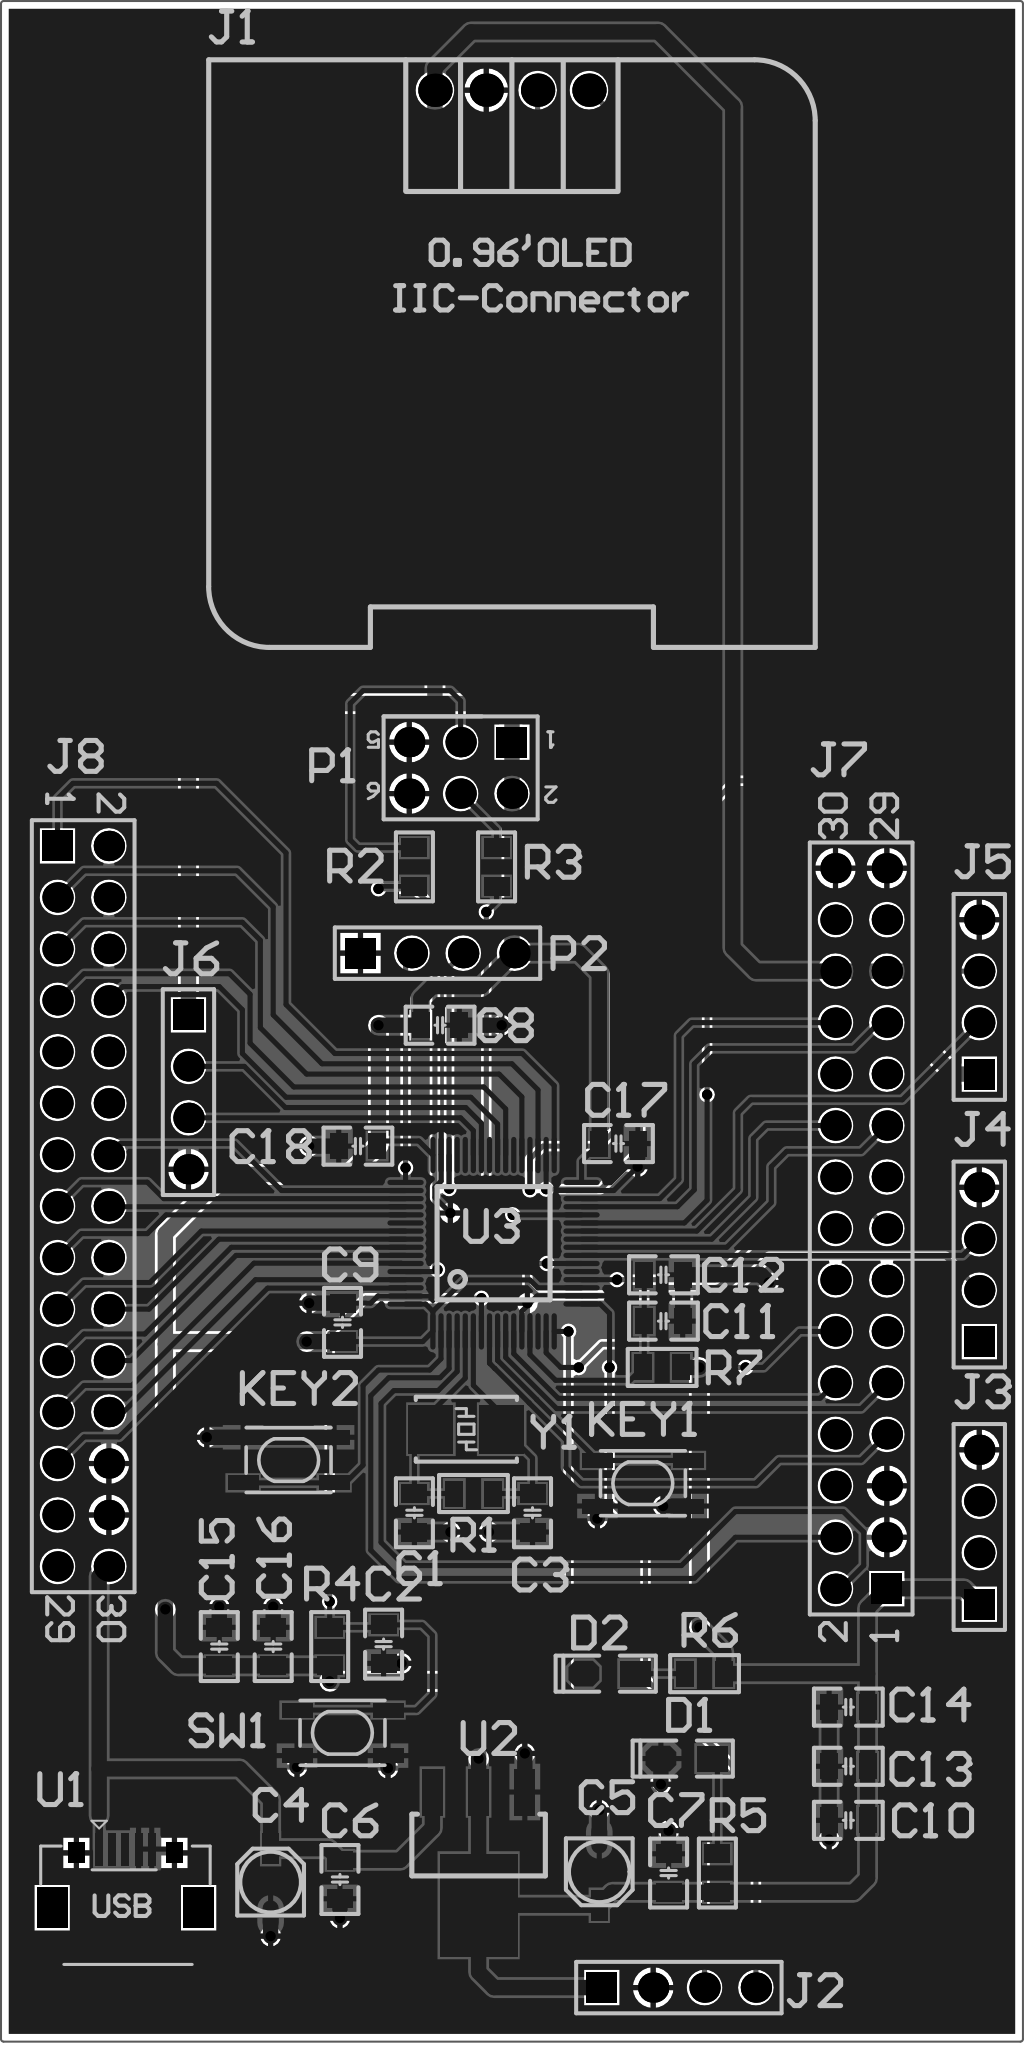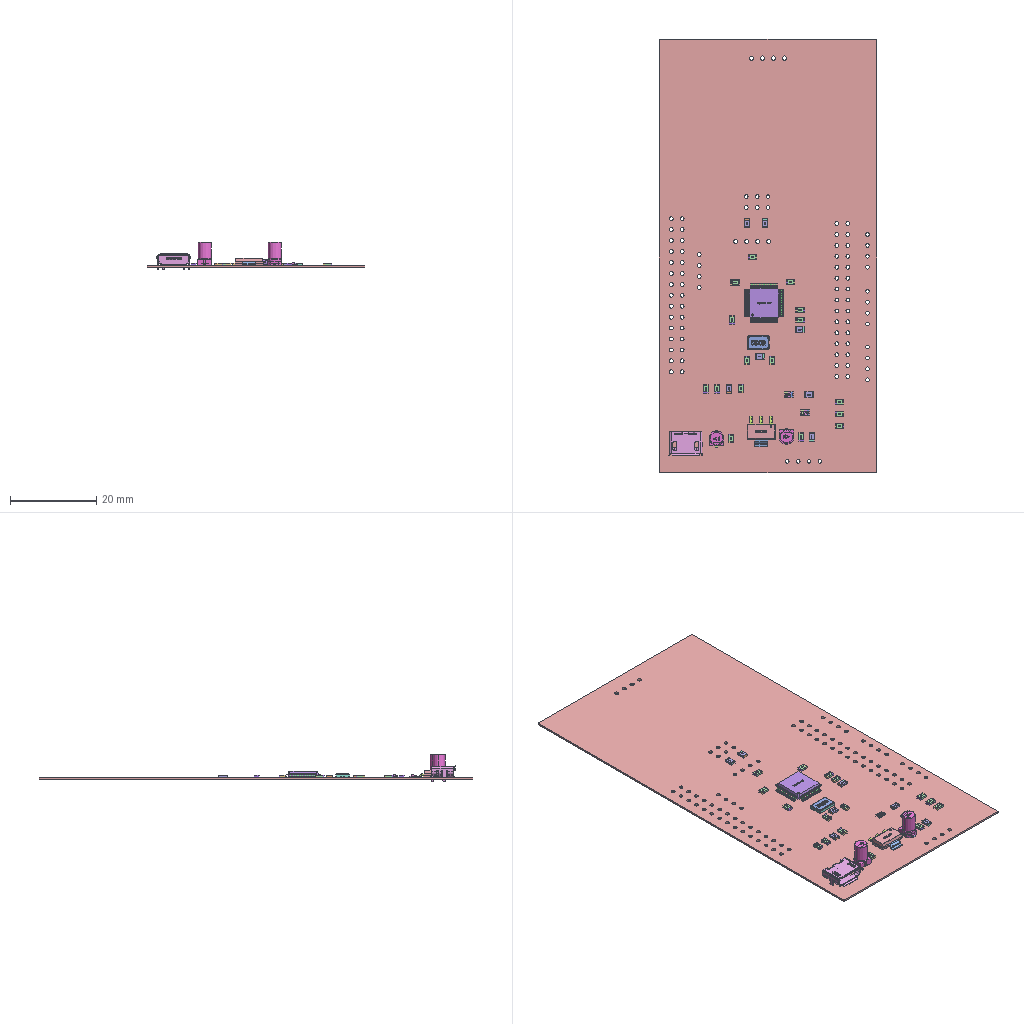Circuit board layout | Altium Designer | box 50.5 x 100.7 x 6.4 mm
Layer stack:
# Altium Designer layer stack of  (unit mm; dielectric type: 0 none, 1 core, 2 prepreg, 3 surface material)
index,name,kind,layer,copper_thickness_mm,dielectric_type,dielectric_thickness_mm,dielectric_material,dielectric_constant
0,Top Paste,other,,,,,,
1,Top Overlay,other,,,,,,
2,Top Solder,dielectric,,,3,0.0102,Solder Resist,3.5
3,Top Layer,copper,Top Layer,0.0356,,,,
4,Dielectric 1,dielectric,,,0,0.32,FR-4,4.8
5,Bottom Layer,copper,Bottom Layer,0.0356,,,,
6,Bottom Solder,dielectric,,,3,0.0102,Solder Resist,3.5
7,Bottom Overlay,other,,,,,,
8,Bottom Paste,other,,,,,,
# drill layer pairs: low layer,high layer
drill_pair,Top Layer,Bottom Layer
Part placement:
Designator,Comment,Layer,Footprint,Center-X(mm),Center-Y(mm),Rotation
Y1,8M,TopLayer,OSC_5032-2P,74.323,63.881,180
U3,STM32F103RCT6,TopLayer,LQFP64_7x7,75.67,73.059,0
U2,AMS1117-3.3,TopLayer,SOT223,74.93,43.18,180
U1,USB-Micro,TopLayer,USB-MICRO_B,57.462,41.709,0
SW1,SW-PB,TopLayer,TSW_SMD-3*4*2.5,68.199,48.895,180
R7,Res2,TopLayer,R_0805_L,84.008,66.929,180
R6,Res1,TopLayer,R_0805_L,86.106,51.816,180
R5,Res1,TopLayer,R_0805_L,86.741,41.976,90
R4,Res2,TopLayer,R_0805_L,67.564,53.152,270
R3,Res2,TopLayer,R_0805_L,75.819,91.633,270
R2,Res2,TopLayer,R_0805_L,71.755,91.633,90
R1,,TopLayer,R_0805_L,74.676,60.706,180
P2,SWD,TopLayer,HDR1X4,72.898,87.376,360
P1,Header 3X2,TopLayer,HDR2X3,74.041,96.52,180
KEY2,SW-PB,TopLayer,TSW_SMD-3*4*2.5,65.532,62.357,360
KEY1,SW-PB,TopLayer,TSW_SMD-3*4*2.5,83.058,61.214,180
J8,HEADER 15X2,TopLayer,HDR2X15,55.372,74.887,270
J7,HEADER 15X2,TopLayer,HDR2X15,93.853,73.787,90
J6,HC-SR04,TopLayer,HDR1X4,60.579,80.518,270
J5,HC-SR04,TopLayer,HDR1X4,99.695,85.217,90
J4,HC-SR04,TopLayer,HDR1X4,99.695,72.009,90
J3,HC-SR04,TopLayer,HDR1X4,99.695,59.055,90
J2,SIM900A,TopLayer,HDR1X4,84.836,36.322,360
J1,OLED,TopLayer,0.96OLED_4P,76.58,129.966,0
D2,LED0,TopLayer,LED_0805G,81.407,51.816,180
D1,LED0,TopLayer,LED_0805G,85.217,47.625,180
C18,Cap,TopLayer,C_0805_L,68.961,77.851,360
C17,Cap,TopLayer,C_0805_L,81.849,77.978,180
C16,Cap,TopLayer,C_0805_L,64.77,53.152,270
C15,Cap,TopLayer,C_0805_L,62.103,53.152,270
C14,Cap,TopLayer,C_0805_L,93.218,50.165,180
C13,Cap,TopLayer,C_0805_L,93.218,47.244,180
C12,Cap,TopLayer,C_0805_L,84.074,71.501,0
C11,Cap,TopLayer,C_0805_L,84.074,69.215,0
C10,Cap,TopLayer,C_0805_L,93.218,44.577,360
C9,Cap,TopLayer,C_0805_L,68.199,69.154,270
C8,Cap,TopLayer,C_0805_L,73.025,83.82,180
C7,Cap,TopLayer,C_0805_L,84.328,41.976,270
C6,Cap,TopLayer,C_0805_L,68.072,41.656,90
C5,Cap Pol1,TopLayer,CM_A(3*5.4),80.899,42.036,270
C4,Cap Pol1,TopLayer,CM_A(3*5.4),64.643,41.529,90
C3,Cap,TopLayer,C_0805_L,77.597,59.756,90
C2,,TopLayer,C_0805_L,70.231,53.274,90
C1,Cap,TopLayer,C_0805_L,71.755,59.756,90
Pad and via stacks:
# Altium Designer via and pad stacks of  (unit mm). Each distinct definition once, with the count of objects using it.
# via: kind,start_layer,end_layer,hole_mm,diameter_mm,mode(0 simple;1 top-mid-bottom;2 full stack),diameter_per_layer,count,example_net
# pad: kind,layer,hole_mm,hole_type(0 round;1 square;2 slot),plating,top_size,top_shape(1 round;2 rect;3 octagon;9 rounded rect),mid_size,bottom_size,mode,footprint,size_per_layer,count,example
pad,Top Layer,0,0,plated,1.5x0.7,2,1.5x0.7,1.5x0.7,0,TSW SMD-3*4*2.5,,12,SW1.1
pad,Top Layer,0,0,plated,1.6x0.35,2,1.6x0.35,1.6x0.35,0,USB-MICRO_B,,5,U1.4
pad,Top Layer,0,0,plated,1.27x0.889,2,1.27x0.889,1.27x0.889,0,C 0805_L,,32,C1.1
pad,Top Layer,0,0,plated,1.27x0.889,2,1.27x0.889,1.27x0.889,0,R 0805_L,,14,R1.1
pad,Top Layer,0,0,unplated,2.4x2.2,2,2.4x2.2,2.4x2.2,0,OSC 5032-2P,,2,Y1.2
pad,Top Layer,0,0,plated,1.524x1.27,2,1.524x1.27,1.524x1.27,0,LED 0805G,,2,D1.1
pad,Top Layer,0,0,plated,1.524x1.27,3,1.524x1.27,1.524x1.27,0,LED 0805G,,2,D1.2
pad,Top Layer,0,0,plated,1.016x2.286,2,1.016x2.286,1.016x2.286,0,SOT223,,3,U2.3
pad,Top Layer,0,0,plated,3.81x5.08,2,3.81x5.08,3.81x5.08,0,SOT223,,1,U2.2
pad,Top Layer,0,0,plated,1.5x0.8,2,1.5x0.8,1.5x0.8,0,CM A(3*5.4),,2,C5.1
pad,Top Layer,0,0,plated,1.5x0.8,1,1.5x0.8,1.5x0.8,0,CM A(3*5.4),,2,C5.2
pad,Top Layer,0,0,plated,0.26x1.8,1,0.26x1.8,0.26x1.8,0,LQFP64 7x7,,64,U3.1
pad,Multi-Layer,0.5,2,plated,1.5x2,2,1.5x2,1.5x2,0,USB-MICRO_B,,2,U1.0
pad,Multi-Layer,0.5,0,plated,0.8x1,2,0.8x1,0.8x1,0,USB-MICRO_B,,2,U1.5
pad,Multi-Layer,1,2,plated,1.65x1.65,1,1.65x1.65,1.65x1.65,0,0.96OLED_4P,,4,J1.4
pad,Multi-Layer,0.9,0,plated,1.5x1.5,2,1.5x1.5,1.5x1.5,0,HDR2X3,,1,P1.1
pad,Multi-Layer,0.9,0,plated,1.5x1.5,1,1.5x1.5,1.5x1.5,0,HDR2X3,,5,P1.2
pad,Multi-Layer,0.9,0,plated,1.5x1.5,1,1.5x1.5,1.5x1.5,0,HDR1X4,,18,J2.4
pad,Multi-Layer,0.9,0,plated,1.5x1.5,2,1.5x1.5,1.5x1.5,0,HDR1X4,,6,J2.1
pad,Multi-Layer,0.9,0,plated,1.5x1.5,1,1.5x1.5,1.5x1.5,0,HDR2X15,,58,J7.30
pad,Multi-Layer,0.9,0,plated,1.5x1.5,2,1.5x1.5,1.5x1.5,0,HDR2X15,,2,J7.1
via,Top Layer,Bottom Layer,0.254,0.508,0,,49,GND
Copper pours:
name,layer,net,type(0 solid;1 hatched;2 none)
D,Bottom Layer,GND,0
D,Top Layer,GND,0
Design rules, without the lines most boards share:
# Altium Designer design rules of  (exported by Altium Designer, unit mm)
# columns: name | kind | enabled | priority | scope1 | scope2 | descriptor | typed fields (field=value)
SilkToSilkClearance | 55 | enabled | 1 | All | All | Silk to Silk (Clearance=0mil) (All),(All) |
SilkToSolderMaskClearance | 54 | enabled | 1 | IsPad | All | Silk To Solder Mask (Clearance=0mil) (IsPad),(All) |
MinimumSolderMaskSliver | 53 | enabled | 1 | All | All | Minimum Solder Mask Sliver (Gap=0mil) (All),(All) |
HoleToHoleClearance | 52 | enabled | 1 | All | All | Hole To Hole Clearance (Gap=10mil) (All),(All) | gap=0.254
DiffPairsRouting | 51 | enabled | 1 | All | All | Differential Pairs Uncoupled Length using the Gap Constraints (Min=10mil) (Max=10mil) (Prefered=10mil)  and Width Constraints (Min=15mil) (Max=15mil) (Prefered=15mil) (All) |
SolderMaskExpansion | 13 | enabled | 1 | All | All | Solder Mask Expansion (Expansion =4mil) (All) | expansion=0.1016
PasteMaskExpansion | 14 | enabled | 1 | All | All | Paste Mask Expansion (Expansion =0mil) (All) | expansion=0
RoutingVias | 11 | enabled | 1 | All | All | Routing Via (MinHoleWidth=28mil) (MaxHoleWidth=28mil) (PreferredHoleWidth=28mil) (MinWidth=50mil) (MaxWidth=50mil) (PreferedWidth=50mil) (All) | via_min_hole=0.7112 via_max_hole=0.7112 via_preferred_diameter=1.27 via_preferred_hole=0.7112
Width | 2 | enabled | 1 | All | All | Width Constraint (Min=10mil) (Max=30mil) (Preferred=10mil) (All) |
PolygonConnect | 20 | enabled | 1 | All | All | Polygon Connect Rule(Relief Connect )(Conductor Width=10mil) (Relief Angle=90 Angle) (Entries=4) (Air Gap Width=10mil) (All),(All) | connect_style(0=relief,1=direct,2=none)=0 relief_conductor_width=0.254 relief_entries=4
PlaneConnect | 6 | enabled | 1 | All | All | Power Plane Connect Rule(Relief Connect )(Expansion=20mil) (Conductor Width=10mil) (Air Gap=10mil) (Entries=4) (All) | relief_conductor_width=0.254 relief_entries=4 relief_expansion=0.508
Clearance | 0 | enabled | 1 | All | All | Clearance Constraint (Gap=5mil) (All),(All) | gap=0.127
Classes set for this board:
# Altium Designer classes of  (member kind: 0 net, 1 component, 2 from-to, 3 pad, 4 layer, 5 differential pair, 6 design channel, 7 polygon, 8 structure, 9 xSignal)
# columns: class name | member kind | superclass | members
STM32F103C8T61 | 1 | no | C1; C2; C3; C4; C5; C6; C7; C8; C9; C10; C11; C12; C13; C14; C15; C16; C17; C18; D1; D2; J1; J2; J3; J4; J5; J6; J7; J8; KEY1; KEY2; P1; P2; R1; R2; R3; R4; R5; R6; R7; SW1; U1; U2; U3; Y1;